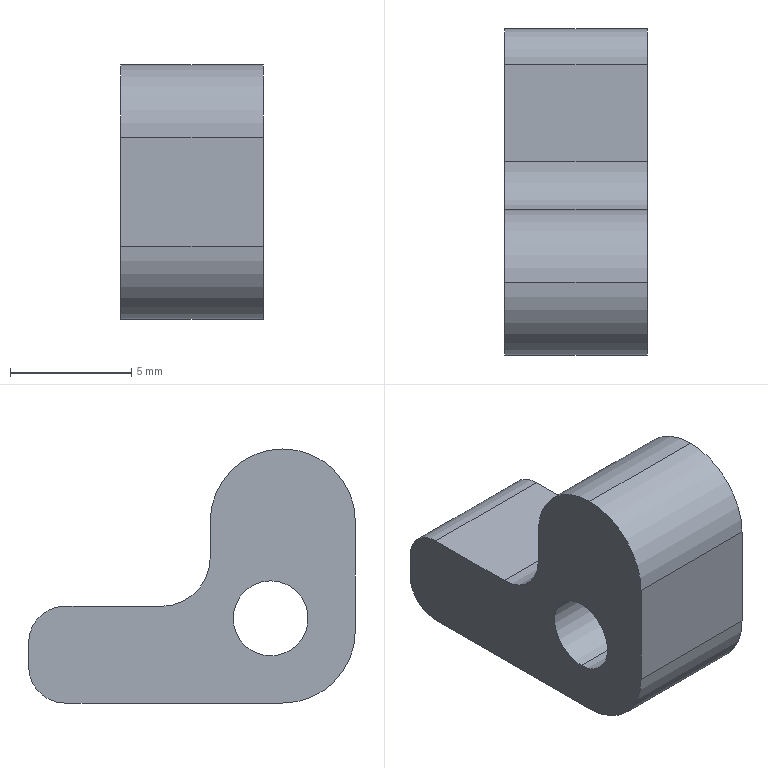Part | STEP file | PN_0095 limit clamp block | 1 solid | 15 faces | box 5.9 x 13.5 x 10.5 mm | volume 469.35 mm3 | cylinder 8 | plane 7 | commonest cylinder face diameters 6 x3 3 x2 3.1 x2 4 x1
STEP:
#1=CARTESIAN_POINT('',(0.,0.,0.));
#2=DIRECTION('',(0.,0.,1.));
#3=DIRECTION('',(1.,0.,0.));
#4=AXIS2_PLACEMENT_3D('',#1,#2,#3);
#5=CARTESIAN_POINT('',(-2.95,0.,1.95));
#6=VERTEX_POINT('',#5);
#7=CARTESIAN_POINT('',(2.95,0.,1.95));
#8=VERTEX_POINT('',#7);
#9=CARTESIAN_POINT('',(-2.95,0.,1.95));
#10=DIRECTION('',(1.,0.,0.));
#11=VECTOR('',#10,1.);
#12=LINE('',#9,#11);
#13=CARTESIAN_POINT('',(-2.95,0.,3.5));
#14=DIRECTION('',(1.,0.,0.));
#15=DIRECTION('',(0.,0.,-1.));
#16=AXIS2_PLACEMENT_3D('',#13,#14,#15);
#17=CYLINDRICAL_SURFACE('',#16,1.55);
#18=CARTESIAN_POINT('',(6.283,0.));
#19=DIRECTION('',(0.,1.));
#20=VECTOR('',#19,1.);
#21=LINE('',#18,#20);
#22=(GEOMETRIC_REPRESENTATION_CONTEXT(2)PARAMETRIC_REPRESENTATION_CONTEXT()REPRESENTATION_CONTEXT('',''));
#23=DEFINITIONAL_REPRESENTATION('',(#21),#22);
#24=PCURVE('',#17,#23);
#25=CARTESIAN_POINT('',(-2.95,0.,3.5));
#26=DIRECTION('',(1.,0.,0.));
#27=DIRECTION('',(0.,0.,-1.));
#28=AXIS2_PLACEMENT_3D('',#25,#26,#27);
#29=CYLINDRICAL_SURFACE('',#28,1.55);
#30=CARTESIAN_POINT('',(0.,0.));
#31=DIRECTION('',(0.,1.));
#32=VECTOR('',#31,1.);
#33=LINE('',#30,#32);
#34=(GEOMETRIC_REPRESENTATION_CONTEXT(2)PARAMETRIC_REPRESENTATION_CONTEXT()REPRESENTATION_CONTEXT('',''));
#35=DEFINITIONAL_REPRESENTATION('',(#33),#34);
#36=PCURVE('',#29,#35);
#37=SURFACE_CURVE('',#12,(#24,#36),.PCURVE_S1.);
#38=EDGE_CURVE('',#6,#8,#37,.T.);
#39=ORIENTED_EDGE('',*,*,#38,.T.);
#40=CARTESIAN_POINT('',(2.95,0.,5.05));
#41=VERTEX_POINT('',#40);
#42=CARTESIAN_POINT('',(2.95,0.,3.5));
#43=DIRECTION('',(1.,0.,0.));
#44=DIRECTION('',(0.,0.,-1.));
#45=AXIS2_PLACEMENT_3D('',#42,#43,#44);
#46=CIRCLE('',#45,1.55);
#47=CARTESIAN_POINT('',(0.,5.9));
#48=DIRECTION('',(1.,0.));
#49=VECTOR('',#48,1.);
#50=LINE('',#47,#49);
#51=(GEOMETRIC_REPRESENTATION_CONTEXT(2)PARAMETRIC_REPRESENTATION_CONTEXT()REPRESENTATION_CONTEXT('',''));
#52=DEFINITIONAL_REPRESENTATION('',(#50),#51);
#53=PCURVE('',#17,#52);
#54=CARTESIAN_POINT('',(2.95,-10.,4.));
#55=DIRECTION('',(-1.,0.,0.));
#56=DIRECTION('',(0.,0.,1.));
#57=AXIS2_PLACEMENT_3D('',#54,#55,#56);
#58=PLANE('',#57);
#59=CARTESIAN_POINT('',(-2.05,10.));
#60=CARTESIAN_POINT('',(-2.05,12.685));
#61=CARTESIAN_POINT('',(0.275,11.342));
#62=CARTESIAN_POINT('',(2.6,10.));
#63=CARTESIAN_POINT('',(0.275,8.658));
#64=CARTESIAN_POINT('',(-2.05,7.315));
#65=CARTESIAN_POINT('',(-2.05,10.));
#66=(BOUNDED_CURVE()B_SPLINE_CURVE(2,(#59,#60,#61,#62,#63,#64,#65),.UNSPECIFIED.,.T.,.F.)B_SPLINE_CURVE_WITH_KNOTS((1,2,2,2,2,1),(-2.094,0.,2.094,4.189,6.283,8.378),.UNSPECIFIED.)CURVE()GEOMETRIC_REPRESENTATION_ITEM()RATIONAL_B_SPLINE_CURVE((1.,0.5,1.,0.5,1.,0.5,1.))REPRESENTATION_ITEM(''));
#67=(GEOMETRIC_REPRESENTATION_CONTEXT(2)PARAMETRIC_REPRESENTATION_CONTEXT()REPRESENTATION_CONTEXT('',''));
#68=DEFINITIONAL_REPRESENTATION('',(#66),#67);
#69=PCURVE('',#58,#68);
#70=SURFACE_CURVE('',#46,(#53,#69),.PCURVE_S1.);
#71=EDGE_CURVE('',#41,#8,#70,.T.);
#72=ORIENTED_EDGE('',*,*,#71,.F.);
#73=CARTESIAN_POINT('',(-2.95,0.,5.05));
#74=VERTEX_POINT('',#73);
#75=CARTESIAN_POINT('',(-2.95,0.,5.05));
#76=DIRECTION('',(1.,0.,0.));
#77=VECTOR('',#76,1.);
#78=LINE('',#75,#77);
#79=CARTESIAN_POINT('',(3.142,0.));
#80=DIRECTION('',(0.,1.));
#81=VECTOR('',#80,1.);
#82=LINE('',#79,#81);
#83=(GEOMETRIC_REPRESENTATION_CONTEXT(2)PARAMETRIC_REPRESENTATION_CONTEXT()REPRESENTATION_CONTEXT('',''));
#84=DEFINITIONAL_REPRESENTATION('',(#82),#83);
#85=PCURVE('',#17,#84);
#86=CARTESIAN_POINT('',(3.142,0.));
#87=DIRECTION('',(0.,1.));
#88=VECTOR('',#87,1.);
#89=LINE('',#86,#88);
#90=(GEOMETRIC_REPRESENTATION_CONTEXT(2)PARAMETRIC_REPRESENTATION_CONTEXT()REPRESENTATION_CONTEXT('',''));
#91=DEFINITIONAL_REPRESENTATION('',(#89),#90);
#92=PCURVE('',#29,#91);
#93=SURFACE_CURVE('',#78,(#85,#92),.PCURVE_S1.);
#94=EDGE_CURVE('',#74,#41,#93,.T.);
#95=ORIENTED_EDGE('',*,*,#94,.F.);
#96=CARTESIAN_POINT('',(-2.95,0.,3.5));
#97=DIRECTION('',(1.,0.,0.));
#98=DIRECTION('',(0.,0.,-1.));
#99=AXIS2_PLACEMENT_3D('',#96,#97,#98);
#100=CIRCLE('',#99,1.55);
#101=CARTESIAN_POINT('',(0.,0.00005));
#102=DIRECTION('',(1.,0.));
#103=VECTOR('',#102,1.);
#104=LINE('',#101,#103);
#105=(GEOMETRIC_REPRESENTATION_CONTEXT(2)PARAMETRIC_REPRESENTATION_CONTEXT()REPRESENTATION_CONTEXT('',''));
#106=DEFINITIONAL_REPRESENTATION('',(#104),#105);
#107=PCURVE('',#17,#106);
#108=CARTESIAN_POINT('',(-2.95,-10.,4.));
#109=DIRECTION('',(1.,0.,0.));
#110=DIRECTION('',(0.,0.,-1.));
#111=AXIS2_PLACEMENT_3D('',#108,#109,#110);
#112=PLANE('',#111);
#113=CARTESIAN_POINT('',(0.5,10.));
#114=DIRECTION('',(1.,0.));
#115=AXIS2_PLACEMENT_2D('',#113,#114);
#116=CIRCLE('',#115,1.55);
#117=(GEOMETRIC_REPRESENTATION_CONTEXT(2)PARAMETRIC_REPRESENTATION_CONTEXT()REPRESENTATION_CONTEXT('',''));
#118=DEFINITIONAL_REPRESENTATION('',(#116),#117);
#119=PCURVE('',#112,#118);
#120=SURFACE_CURVE('',#100,(#107,#119),.PCURVE_S1.);
#121=EDGE_CURVE('',#74,#6,#120,.T.);
#122=ORIENTED_EDGE('',*,*,#121,.T.);
#123=EDGE_LOOP('',(#39,#72,#95,#122));
#124=FACE_BOUND('',#123,.F.);
#125=ADVANCED_FACE('',(#124),#17,.F.);
#126=CARTESIAN_POINT('',(2.95,0.,3.5));
#127=DIRECTION('',(1.,0.,0.));
#128=DIRECTION('',(0.,0.,-1.));
#129=AXIS2_PLACEMENT_3D('',#126,#127,#128);
#130=CIRCLE('',#129,1.55);
#131=CARTESIAN_POINT('',(-2.05,10.));
#132=CARTESIAN_POINT('',(-2.05,12.685));
#133=CARTESIAN_POINT('',(0.275,11.342));
#134=CARTESIAN_POINT('',(2.6,10.));
#135=CARTESIAN_POINT('',(0.275,8.658));
#136=CARTESIAN_POINT('',(-2.05,7.315));
#137=CARTESIAN_POINT('',(-2.05,10.));
#138=(BOUNDED_CURVE()B_SPLINE_CURVE(2,(#131,#132,#133,#134,#135,#136,#137),.UNSPECIFIED.,.T.,.F.)B_SPLINE_CURVE_WITH_KNOTS((1,2,2,2,2,1),(-2.094,0.,2.094,4.189,6.283,8.378),.UNSPECIFIED.)CURVE()GEOMETRIC_REPRESENTATION_ITEM()RATIONAL_B_SPLINE_CURVE((1.,0.5,1.,0.5,1.,0.5,1.))REPRESENTATION_ITEM(''));
#139=(GEOMETRIC_REPRESENTATION_CONTEXT(2)PARAMETRIC_REPRESENTATION_CONTEXT()REPRESENTATION_CONTEXT('',''));
#140=DEFINITIONAL_REPRESENTATION('',(#138),#139);
#141=PCURVE('',#58,#140);
#142=CARTESIAN_POINT('',(0.,5.9));
#143=DIRECTION('',(1.,0.));
#144=VECTOR('',#143,1.);
#145=LINE('',#142,#144);
#146=(GEOMETRIC_REPRESENTATION_CONTEXT(2)PARAMETRIC_REPRESENTATION_CONTEXT()REPRESENTATION_CONTEXT('',''));
#147=DEFINITIONAL_REPRESENTATION('',(#145),#146);
#148=PCURVE('',#29,#147);
#149=SURFACE_CURVE('',#130,(#141,#148),.PCURVE_S1.);
#150=EDGE_CURVE('',#8,#41,#149,.T.);
#151=ORIENTED_EDGE('',*,*,#150,.F.);
#152=ORIENTED_EDGE('',*,*,#71,.F.);
#153=EDGE_LOOP('',(#151,#152));
#154=FACE_BOUND('',#153,.T.);
#155=CARTESIAN_POINT('',(2.95,2.5,7.5));
#156=VERTEX_POINT('',#155);
#157=CARTESIAN_POINT('',(2.95,-0.5,10.5));
#158=VERTEX_POINT('',#157);
#159=CARTESIAN_POINT('',(2.95,-0.5,7.5));
#160=DIRECTION('',(1.,0.,0.));
#161=DIRECTION('',(0.,0.,1.));
#162=AXIS2_PLACEMENT_3D('',#159,#160,#161);
#163=CIRCLE('',#162,3.);
#164=CARTESIAN_POINT('',(6.5,9.5));
#165=CARTESIAN_POINT('',(6.5,4.304));
#166=CARTESIAN_POINT('',(2.,6.902));
#167=CARTESIAN_POINT('',(-2.5,9.5));
#168=CARTESIAN_POINT('',(2.,12.098));
#169=CARTESIAN_POINT('',(6.5,14.696));
#170=CARTESIAN_POINT('',(6.5,9.5));
#171=(BOUNDED_CURVE()B_SPLINE_CURVE(2,(#164,#165,#166,#167,#168,#169,#170),.UNSPECIFIED.,.T.,.F.)B_SPLINE_CURVE_WITH_KNOTS((1,2,2,2,2,1),(-2.094,0.,2.094,4.189,6.283,8.378),.UNSPECIFIED.)CURVE()GEOMETRIC_REPRESENTATION_ITEM()RATIONAL_B_SPLINE_CURVE((1.,0.5,1.,0.5,1.,0.5,1.))REPRESENTATION_ITEM(''));
#172=(GEOMETRIC_REPRESENTATION_CONTEXT(2)PARAMETRIC_REPRESENTATION_CONTEXT()REPRESENTATION_CONTEXT('',''));
#173=DEFINITIONAL_REPRESENTATION('',(#171),#172);
#174=PCURVE('',#58,#173);
#175=CARTESIAN_POINT('',(0.,-0.5,7.5));
#176=DIRECTION('',(-1.,0.,0.));
#177=DIRECTION('',(0.,0.,1.));
#178=AXIS2_PLACEMENT_3D('',#175,#176,#177);
#179=CYLINDRICAL_SURFACE('',#178,3.);
#180=CARTESIAN_POINT('',(6.283,-2.95));
#181=DIRECTION('',(-1.,0.));
#182=VECTOR('',#181,1.);
#183=LINE('',#180,#182);
#184=(GEOMETRIC_REPRESENTATION_CONTEXT(2)PARAMETRIC_REPRESENTATION_CONTEXT()REPRESENTATION_CONTEXT('',''));
#185=DEFINITIONAL_REPRESENTATION('',(#183),#184);
#186=PCURVE('',#179,#185);
#187=SURFACE_CURVE('',#163,(#174,#186),.PCURVE_S1.);
#188=EDGE_CURVE('',#156,#158,#187,.T.);
#189=ORIENTED_EDGE('',*,*,#188,.T.);
#190=CARTESIAN_POINT('',(2.95,-3.5,7.5));
#191=VERTEX_POINT('',#190);
#192=CARTESIAN_POINT('',(2.95,-0.5,7.5));
#193=DIRECTION('',(1.,0.,0.));
#194=DIRECTION('',(0.,0.,1.));
#195=AXIS2_PLACEMENT_3D('',#192,#193,#194);
#196=CIRCLE('',#195,3.);
#197=CARTESIAN_POINT('',(6.5,9.5));
#198=CARTESIAN_POINT('',(6.5,4.304));
#199=CARTESIAN_POINT('',(2.,6.902));
#200=CARTESIAN_POINT('',(-2.5,9.5));
#201=CARTESIAN_POINT('',(2.,12.098));
#202=CARTESIAN_POINT('',(6.5,14.696));
#203=CARTESIAN_POINT('',(6.5,9.5));
#204=(BOUNDED_CURVE()B_SPLINE_CURVE(2,(#197,#198,#199,#200,#201,#202,#203),.UNSPECIFIED.,.T.,.F.)B_SPLINE_CURVE_WITH_KNOTS((1,2,2,2,2,1),(-2.094,0.,2.094,4.189,6.283,8.378),.UNSPECIFIED.)CURVE()GEOMETRIC_REPRESENTATION_ITEM()RATIONAL_B_SPLINE_CURVE((1.,0.5,1.,0.5,1.,0.5,1.))REPRESENTATION_ITEM(''));
#205=(GEOMETRIC_REPRESENTATION_CONTEXT(2)PARAMETRIC_REPRESENTATION_CONTEXT()REPRESENTATION_CONTEXT('',''));
#206=DEFINITIONAL_REPRESENTATION('',(#204),#205);
#207=PCURVE('',#58,#206);
#208=CARTESIAN_POINT('',(0.,-0.5,7.5));
#209=DIRECTION('',(1.,0.,0.));
#210=DIRECTION('',(0.,0.,-1.));
#211=AXIS2_PLACEMENT_3D('',#208,#209,#210);
#212=CYLINDRICAL_SURFACE('',#211,3.);
#213=CARTESIAN_POINT('',(3.142,2.95));
#214=DIRECTION('',(1.,0.));
#215=VECTOR('',#214,1.);
#216=LINE('',#213,#215);
#217=(GEOMETRIC_REPRESENTATION_CONTEXT(2)PARAMETRIC_REPRESENTATION_CONTEXT()REPRESENTATION_CONTEXT('',''));
#218=DEFINITIONAL_REPRESENTATION('',(#216),#217);
#219=PCURVE('',#212,#218);
#220=SURFACE_CURVE('',#196,(#207,#219),.PCURVE_S1.);
#221=EDGE_CURVE('',#158,#191,#220,.T.);
#222=ORIENTED_EDGE('',*,*,#221,.T.);
#223=CARTESIAN_POINT('',(2.95,-3.5,3.));
#224=VERTEX_POINT('',#223);
#225=CARTESIAN_POINT('',(2.95,-3.5,10.5));
#226=DIRECTION('',(0.,0.,-1.));
#227=VECTOR('',#226,1.);
#228=LINE('',#225,#227);
#229=CARTESIAN_POINT('',(6.5,6.5));
#230=DIRECTION('',(-1.,0.));
#231=VECTOR('',#230,1.);
#232=LINE('',#229,#231);
#233=(GEOMETRIC_REPRESENTATION_CONTEXT(2)PARAMETRIC_REPRESENTATION_CONTEXT()REPRESENTATION_CONTEXT('',''));
#234=DEFINITIONAL_REPRESENTATION('',(#232),#233);
#235=PCURVE('',#58,#234);
#236=CARTESIAN_POINT('',(-2.95,-3.5,10.5));
#237=DIRECTION('',(0.,1.,0.));
#238=DIRECTION('',(0.,0.,1.));
#239=AXIS2_PLACEMENT_3D('',#236,#237,#238);
#240=PLANE('',#239);
#241=CARTESIAN_POINT('',(0.,5.9));
#242=DIRECTION('',(-1.,0.));
#243=VECTOR('',#242,1.);
#244=LINE('',#241,#243);
#245=(GEOMETRIC_REPRESENTATION_CONTEXT(2)PARAMETRIC_REPRESENTATION_CONTEXT()REPRESENTATION_CONTEXT('',''));
#246=DEFINITIONAL_REPRESENTATION('',(#244),#245);
#247=PCURVE('',#240,#246);
#248=SURFACE_CURVE('',#228,(#235,#247),.PCURVE_S1.);
#249=EDGE_CURVE('',#191,#224,#248,.T.);
#250=ORIENTED_EDGE('',*,*,#249,.T.);
#251=CARTESIAN_POINT('',(2.95,-0.5,0.));
#252=VERTEX_POINT('',#251);
#253=CARTESIAN_POINT('',(2.95,-0.5,3.));
#254=DIRECTION('',(1.,0.,0.));
#255=DIRECTION('',(0.,0.,1.));
#256=AXIS2_PLACEMENT_3D('',#253,#254,#255);
#257=CIRCLE('',#256,3.);
#258=CARTESIAN_POINT('',(2.,9.5));
#259=CARTESIAN_POINT('',(2.,4.304));
#260=CARTESIAN_POINT('',(-2.5,6.902));
#261=CARTESIAN_POINT('',(-7.,9.5));
#262=CARTESIAN_POINT('',(-2.5,12.098));
#263=CARTESIAN_POINT('',(2.,14.696));
#264=CARTESIAN_POINT('',(2.,9.5));
#265=(BOUNDED_CURVE()B_SPLINE_CURVE(2,(#258,#259,#260,#261,#262,#263,#264),.UNSPECIFIED.,.T.,.F.)B_SPLINE_CURVE_WITH_KNOTS((1,2,2,2,2,1),(-2.094,0.,2.094,4.189,6.283,8.378),.UNSPECIFIED.)CURVE()GEOMETRIC_REPRESENTATION_ITEM()RATIONAL_B_SPLINE_CURVE((1.,0.5,1.,0.5,1.,0.5,1.))REPRESENTATION_ITEM(''));
#266=(GEOMETRIC_REPRESENTATION_CONTEXT(2)PARAMETRIC_REPRESENTATION_CONTEXT()REPRESENTATION_CONTEXT('',''));
#267=DEFINITIONAL_REPRESENTATION('',(#265),#266);
#268=PCURVE('',#58,#267);
#269=CARTESIAN_POINT('',(0.,-0.5,3.));
#270=DIRECTION('',(1.,0.,0.));
#271=DIRECTION('',(0.,0.,-1.));
#272=AXIS2_PLACEMENT_3D('',#269,#270,#271);
#273=CYLINDRICAL_SURFACE('',#272,3.);
#274=CARTESIAN_POINT('',(3.142,2.95));
#275=DIRECTION('',(1.,0.));
#276=VECTOR('',#275,1.);
#277=LINE('',#274,#276);
#278=(GEOMETRIC_REPRESENTATION_CONTEXT(2)PARAMETRIC_REPRESENTATION_CONTEXT()REPRESENTATION_CONTEXT('',''));
#279=DEFINITIONAL_REPRESENTATION('',(#277),#278);
#280=PCURVE('',#273,#279);
#281=SURFACE_CURVE('',#257,(#268,#280),.PCURVE_S1.);
#282=EDGE_CURVE('',#224,#252,#281,.T.);
#283=ORIENTED_EDGE('',*,*,#282,.T.);
#284=CARTESIAN_POINT('',(2.95,8.5,0.));
#285=VERTEX_POINT('',#284);
#286=CARTESIAN_POINT('',(2.95,-10.,0.));
#287=DIRECTION('',(0.,1.,0.));
#288=VECTOR('',#287,1.);
#289=LINE('',#286,#288);
#290=CARTESIAN_POINT('',(-4.,0.));
#291=DIRECTION('',(0.,1.));
#292=VECTOR('',#291,1.);
#293=LINE('',#290,#292);
#294=(GEOMETRIC_REPRESENTATION_CONTEXT(2)PARAMETRIC_REPRESENTATION_CONTEXT()REPRESENTATION_CONTEXT('',''));
#295=DEFINITIONAL_REPRESENTATION('',(#293),#294);
#296=PCURVE('',#58,#295);
#297=CARTESIAN_POINT('',(0.,0.,0.));
#298=DIRECTION('',(0.,0.,-1.));
#299=DIRECTION('',(-1.,0.,0.));
#300=AXIS2_PLACEMENT_3D('',#297,#298,#299);
#301=PLANE('',#300);
#302=CARTESIAN_POINT('',(-2.95,-10.));
#303=DIRECTION('',(0.,1.));
#304=VECTOR('',#303,1.);
#305=LINE('',#302,#304);
#306=(GEOMETRIC_REPRESENTATION_CONTEXT(2)PARAMETRIC_REPRESENTATION_CONTEXT()REPRESENTATION_CONTEXT('',''));
#307=DEFINITIONAL_REPRESENTATION('',(#305),#306);
#308=PCURVE('',#301,#307);
#309=SURFACE_CURVE('',#289,(#296,#308),.PCURVE_S1.);
#310=EDGE_CURVE('',#252,#285,#309,.T.);
#311=ORIENTED_EDGE('',*,*,#310,.T.);
#312=CARTESIAN_POINT('',(2.95,10.,1.5));
#313=VERTEX_POINT('',#312);
#314=CARTESIAN_POINT('',(2.95,8.5,1.5));
#315=DIRECTION('',(1.,0.,0.));
#316=DIRECTION('',(0.,0.,1.));
#317=AXIS2_PLACEMENT_3D('',#314,#315,#316);
#318=CIRCLE('',#317,1.5);
#319=CARTESIAN_POINT('',(-1.,18.5));
#320=CARTESIAN_POINT('',(-1.,15.902));
#321=CARTESIAN_POINT('',(-3.25,17.201));
#322=CARTESIAN_POINT('',(-5.5,18.5));
#323=CARTESIAN_POINT('',(-3.25,19.799));
#324=CARTESIAN_POINT('',(-1.,21.098));
#325=CARTESIAN_POINT('',(-1.,18.5));
#326=(BOUNDED_CURVE()B_SPLINE_CURVE(2,(#319,#320,#321,#322,#323,#324,#325),.UNSPECIFIED.,.T.,.F.)B_SPLINE_CURVE_WITH_KNOTS((1,2,2,2,2,1),(-2.094,0.,2.094,4.189,6.283,8.378),.UNSPECIFIED.)CURVE()GEOMETRIC_REPRESENTATION_ITEM()RATIONAL_B_SPLINE_CURVE((1.,0.5,1.,0.5,1.,0.5,1.))REPRESENTATION_ITEM(''));
#327=(GEOMETRIC_REPRESENTATION_CONTEXT(2)PARAMETRIC_REPRESENTATION_CONTEXT()REPRESENTATION_CONTEXT('',''));
#328=DEFINITIONAL_REPRESENTATION('',(#326),#327);
#329=PCURVE('',#58,#328);
#330=CARTESIAN_POINT('',(-2.95,8.5,1.5));
#331=DIRECTION('',(1.,0.,0.));
#332=DIRECTION('',(0.,0.,-1.));
#333=AXIS2_PLACEMENT_3D('',#330,#331,#332);
#334=CYLINDRICAL_SURFACE('',#333,1.5);
#335=CARTESIAN_POINT('',(-3.142,5.9));
#336=DIRECTION('',(1.,0.));
#337=VECTOR('',#336,1.);
#338=LINE('',#335,#337);
#339=(GEOMETRIC_REPRESENTATION_CONTEXT(2)PARAMETRIC_REPRESENTATION_CONTEXT()REPRESENTATION_CONTEXT('',''));
#340=DEFINITIONAL_REPRESENTATION('',(#338),#339);
#341=PCURVE('',#334,#340);
#342=SURFACE_CURVE('',#318,(#329,#341),.PCURVE_S1.);
#343=EDGE_CURVE('',#285,#313,#342,.T.);
#344=ORIENTED_EDGE('',*,*,#343,.T.);
#345=CARTESIAN_POINT('',(2.95,10.,2.5));
#346=VERTEX_POINT('',#345);
#347=CARTESIAN_POINT('',(2.95,10.,4.));
#348=DIRECTION('',(0.,0.,-1.));
#349=VECTOR('',#348,1.);
#350=LINE('',#347,#349);
#351=CARTESIAN_POINT('',(0.,20.));
#352=DIRECTION('',(-1.,0.));
#353=VECTOR('',#352,1.);
#354=LINE('',#351,#353);
#355=(GEOMETRIC_REPRESENTATION_CONTEXT(2)PARAMETRIC_REPRESENTATION_CONTEXT()REPRESENTATION_CONTEXT('',''));
#356=DEFINITIONAL_REPRESENTATION('',(#354),#355);
#357=PCURVE('',#58,#356);
#358=CARTESIAN_POINT('',(-2.95,10.,4.));
#359=DIRECTION('',(0.,-1.,0.));
#360=DIRECTION('',(0.,0.,-1.));
#361=AXIS2_PLACEMENT_3D('',#358,#359,#360);
#362=PLANE('',#361);
#363=CARTESIAN_POINT('',(0.,5.9));
#364=DIRECTION('',(1.,0.));
#365=VECTOR('',#364,1.);
#366=LINE('',#363,#365);
#367=(GEOMETRIC_REPRESENTATION_CONTEXT(2)PARAMETRIC_REPRESENTATION_CONTEXT()REPRESENTATION_CONTEXT('',''));
#368=DEFINITIONAL_REPRESENTATION('',(#366),#367);
#369=PCURVE('',#362,#368);
#370=SURFACE_CURVE('',#350,(#357,#369),.PCURVE_S1.);
#371=EDGE_CURVE('',#346,#313,#370,.T.);
#372=ORIENTED_EDGE('',*,*,#371,.F.);
#373=CARTESIAN_POINT('',(2.95,8.5,4.));
#374=VERTEX_POINT('',#373);
#375=CARTESIAN_POINT('',(2.95,8.5,2.5));
#376=DIRECTION('',(1.,0.,0.));
#377=DIRECTION('',(0.,0.,1.));
#378=AXIS2_PLACEMENT_3D('',#375,#376,#377);
#379=CIRCLE('',#378,1.5);
#380=CARTESIAN_POINT('',(0.,18.5));
#381=CARTESIAN_POINT('',(0.,15.902));
#382=CARTESIAN_POINT('',(-2.25,17.201));
#383=CARTESIAN_POINT('',(-4.5,18.5));
#384=CARTESIAN_POINT('',(-2.25,19.799));
#385=CARTESIAN_POINT('',(0.,21.098));
#386=CARTESIAN_POINT('',(0.,18.5));
#387=(BOUNDED_CURVE()B_SPLINE_CURVE(2,(#380,#381,#382,#383,#384,#385,#386),.UNSPECIFIED.,.T.,.F.)B_SPLINE_CURVE_WITH_KNOTS((1,2,2,2,2,1),(-2.094,0.,2.094,4.189,6.283,8.378),.UNSPECIFIED.)CURVE()GEOMETRIC_REPRESENTATION_ITEM()RATIONAL_B_SPLINE_CURVE((1.,0.5,1.,0.5,1.,0.5,1.))REPRESENTATION_ITEM(''));
#388=(GEOMETRIC_REPRESENTATION_CONTEXT(2)PARAMETRIC_REPRESENTATION_CONTEXT()REPRESENTATION_CONTEXT('',''));
#389=DEFINITIONAL_REPRESENTATION('',(#387),#388);
#390=PCURVE('',#58,#389);
#391=CARTESIAN_POINT('',(0.,8.5,2.5));
#392=DIRECTION('',(-1.,0.,0.));
#393=DIRECTION('',(0.,0.,1.));
#394=AXIS2_PLACEMENT_3D('',#391,#392,#393);
#395=CYLINDRICAL_SURFACE('',#394,1.5);
#396=CARTESIAN_POINT('',(6.283,-2.95));
#397=DIRECTION('',(-1.,0.));
#398=VECTOR('',#397,1.);
#399=LINE('',#396,#398);
#400=(GEOMETRIC_REPRESENTATION_CONTEXT(2)PARAMETRIC_REPRESENTATION_CONTEXT()REPRESENTATION_CONTEXT('',''));
#401=DEFINITIONAL_REPRESENTATION('',(#399),#400);
#402=PCURVE('',#395,#401);
#403=SURFACE_CURVE('',#379,(#390,#402),.PCURVE_S1.);
#404=EDGE_CURVE('',#346,#374,#403,.T.);
#405=ORIENTED_EDGE('',*,*,#404,.T.);
#406=CARTESIAN_POINT('',(2.95,4.5,4.));
#407=VERTEX_POINT('',#406);
#408=CARTESIAN_POINT('',(2.95,-10.,4.));
#409=DIRECTION('',(0.,1.,0.));
#410=VECTOR('',#409,1.);
#411=LINE('',#408,#410);
#412=CARTESIAN_POINT('',(0.,0.));
#413=DIRECTION('',(0.,1.));
#414=VECTOR('',#413,1.);
#415=LINE('',#412,#414);
#416=(GEOMETRIC_REPRESENTATION_CONTEXT(2)PARAMETRIC_REPRESENTATION_CONTEXT()REPRESENTATION_CONTEXT('',''));
#417=DEFINITIONAL_REPRESENTATION('',(#415),#416);
#418=PCURVE('',#58,#417);
#419=CARTESIAN_POINT('',(0.,0.,4.));
#420=DIRECTION('',(0.,0.,-1.));
#421=DIRECTION('',(-1.,0.,0.));
#422=AXIS2_PLACEMENT_3D('',#419,#420,#421);
#423=PLANE('',#422);
#424=CARTESIAN_POINT('',(-2.95,-10.));
#425=DIRECTION('',(0.,1.));
#426=VECTOR('',#425,1.);
#427=LINE('',#424,#426);
#428=(GEOMETRIC_REPRESENTATION_CONTEXT(2)PARAMETRIC_REPRESENTATION_CONTEXT()REPRESENTATION_CONTEXT('',''));
#429=DEFINITIONAL_REPRESENTATION('',(#427),#428);
#430=PCURVE('',#423,#429);
#431=SURFACE_CURVE('',#411,(#418,#430),.PCURVE_S1.);
#432=EDGE_CURVE('',#407,#374,#431,.T.);
#433=ORIENTED_EDGE('',*,*,#432,.F.);
#434=CARTESIAN_POINT('',(2.95,2.5,6.));
#435=VERTEX_POINT('',#434);
#436=CARTESIAN_POINT('',(2.95,4.5,6.));
#437=DIRECTION('',(-1.,0.,0.));
#438=DIRECTION('',(0.,0.,1.));
#439=AXIS2_PLACEMENT_3D('',#436,#437,#438);
#440=CIRCLE('',#439,2.);
#441=CARTESIAN_POINT('',(2.,14.5));
#442=DIRECTION('',(1.,0.));
#443=AXIS2_PLACEMENT_2D('',#441,#442);
#444=CIRCLE('',#443,2.);
#445=(GEOMETRIC_REPRESENTATION_CONTEXT(2)PARAMETRIC_REPRESENTATION_CONTEXT()REPRESENTATION_CONTEXT('',''));
#446=DEFINITIONAL_REPRESENTATION('',(#444),#445);
#447=PCURVE('',#58,#446);
#448=CARTESIAN_POINT('',(-2.95,4.5,6.));
#449=DIRECTION('',(1.,0.,0.));
#450=DIRECTION('',(0.,0.,-1.));
#451=AXIS2_PLACEMENT_3D('',#448,#449,#450);
#452=CYLINDRICAL_SURFACE('',#451,2.);
#453=CARTESIAN_POINT('',(9.425,5.9));
#454=DIRECTION('',(-1.,0.));
#455=VECTOR('',#454,1.);
#456=LINE('',#453,#455);
#457=(GEOMETRIC_REPRESENTATION_CONTEXT(2)PARAMETRIC_REPRESENTATION_CONTEXT()REPRESENTATION_CONTEXT('',''));
#458=DEFINITIONAL_REPRESENTATION('',(#456),#457);
#459=PCURVE('',#452,#458);
#460=SURFACE_CURVE('',#440,(#447,#459),.PCURVE_S1.);
#461=EDGE_CURVE('',#407,#435,#460,.T.);
#462=ORIENTED_EDGE('',*,*,#461,.T.);
#463=CARTESIAN_POINT('',(2.95,2.5,10.5));
#464=DIRECTION('',(0.,0.,-1.));
#465=VECTOR('',#464,1.);
#466=LINE('',#463,#465);
#467=CARTESIAN_POINT('',(6.5,12.5));
#468=DIRECTION('',(-1.,0.));
#469=VECTOR('',#468,1.);
#470=LINE('',#467,#469);
#471=(GEOMETRIC_REPRESENTATION_CONTEXT(2)PARAMETRIC_REPRESENTATION_CONTEXT()REPRESENTATION_CONTEXT('',''));
#472=DEFINITIONAL_REPRESENTATION('',(#470),#471);
#473=PCURVE('',#58,#472);
#474=CARTESIAN_POINT('',(-2.95,2.5,10.5));
#475=DIRECTION('',(0.,-1.,0.));
#476=DIRECTION('',(0.,0.,-1.));
#477=AXIS2_PLACEMENT_3D('',#474,#475,#476);
#478=PLANE('',#477);
#479=CARTESIAN_POINT('',(0.,5.9));
#480=DIRECTION('',(1.,0.));
#481=VECTOR('',#480,1.);
#482=LINE('',#479,#481);
#483=(GEOMETRIC_REPRESENTATION_CONTEXT(2)PARAMETRIC_REPRESENTATION_CONTEXT()REPRESENTATION_CONTEXT('',''));
#484=DEFINITIONAL_REPRESENTATION('',(#482),#483);
#485=PCURVE('',#478,#484);
#486=SURFACE_CURVE('',#466,(#473,#485),.PCURVE_S1.);
#487=EDGE_CURVE('',#156,#435,#486,.T.);
#488=ORIENTED_EDGE('',*,*,#487,.F.);
#489=EDGE_LOOP('',(#189,#222,#250,#283,#311,#344,#372,#405,#433,#462,#488));
#490=FACE_BOUND('',#489,.T.);
#491=ADVANCED_FACE('',(#154,#490),#58,.F.);
#492=CARTESIAN_POINT('',(-2.95,0.,3.5));
#493=DIRECTION('',(1.,0.,0.));
#494=DIRECTION('',(0.,0.,-1.));
#495=AXIS2_PLACEMENT_3D('',#492,#493,#494);
#496=CIRCLE('',#495,1.55);
#497=CARTESIAN_POINT('',(0.5,10.));
#498=DIRECTION('',(1.,0.));
#499=AXIS2_PLACEMENT_2D('',#497,#498);
#500=CIRCLE('',#499,1.55);
#501=(GEOMETRIC_REPRESENTATION_CONTEXT(2)PARAMETRIC_REPRESENTATION_CONTEXT()REPRESENTATION_CONTEXT('',''));
#502=DEFINITIONAL_REPRESENTATION('',(#500),#501);
#503=PCURVE('',#112,#502);
#504=CARTESIAN_POINT('',(0.,0.00005));
#505=DIRECTION('',(1.,0.));
#506=VECTOR('',#505,1.);
#507=LINE('',#504,#506);
#508=(GEOMETRIC_REPRESENTATION_CONTEXT(2)PARAMETRIC_REPRESENTATION_CONTEXT()REPRESENTATION_CONTEXT('',''));
#509=DEFINITIONAL_REPRESENTATION('',(#507),#508);
#510=PCURVE('',#29,#509);
#511=SURFACE_CURVE('',#496,(#503,#510),.PCURVE_S1.);
#512=EDGE_CURVE('',#6,#74,#511,.T.);
#513=ORIENTED_EDGE('',*,*,#512,.T.);
#514=ORIENTED_EDGE('',*,*,#121,.T.);
#515=EDGE_LOOP('',(#513,#514));
#516=FACE_BOUND('',#515,.T.);
#517=CARTESIAN_POINT('',(-2.95,-3.5,7.5));
#518=VERTEX_POINT('',#517);
#519=CARTESIAN_POINT('',(-2.95,-3.5,3.));
#520=VERTEX_POINT('',#519);
#521=CARTESIAN_POINT('',(-2.95,-3.5,10.5));
#522=DIRECTION('',(0.,0.,-1.));
#523=VECTOR('',#522,1.);
#524=LINE('',#521,#523);
#525=CARTESIAN_POINT('',(-6.5,6.5));
#526=DIRECTION('',(1.,0.));
#527=VECTOR('',#526,1.);
#528=LINE('',#525,#527);
#529=(GEOMETRIC_REPRESENTATION_CONTEXT(2)PARAMETRIC_REPRESENTATION_CONTEXT()REPRESENTATION_CONTEXT('',''));
#530=DEFINITIONAL_REPRESENTATION('',(#528),#529);
#531=PCURVE('',#112,#530);
#532=CARTESIAN_POINT('',(0.,0.));
#533=DIRECTION('',(-1.,0.));
#534=VECTOR('',#533,1.);
#535=LINE('',#532,#534);
#536=(GEOMETRIC_REPRESENTATION_CONTEXT(2)PARAMETRIC_REPRESENTATION_CONTEXT()REPRESENTATION_CONTEXT('',''));
#537=DEFINITIONAL_REPRESENTATION('',(#535),#536);
#538=PCURVE('',#240,#537);
#539=SURFACE_CURVE('',#524,(#531,#538),.PCURVE_S1.);
#540=EDGE_CURVE('',#518,#520,#539,.T.);
#541=ORIENTED_EDGE('',*,*,#540,.F.);
#542=CARTESIAN_POINT('',(-2.95,-0.5,10.5));
#543=VERTEX_POINT('',#542);
#544=CARTESIAN_POINT('',(-2.95,-0.5,7.5));
#545=DIRECTION('',(-1.,0.,0.));
#546=DIRECTION('',(0.,0.,-1.));
#547=AXIS2_PLACEMENT_3D('',#544,#545,#546);
#548=CIRCLE('',#547,3.);
#549=CARTESIAN_POINT('',(-0.5,9.5));
#550=CARTESIAN_POINT('',(-0.5,4.304));
#551=CARTESIAN_POINT('',(-5.,6.902));
#552=CARTESIAN_POINT('',(-9.5,9.5));
#553=CARTESIAN_POINT('',(-5.,12.098));
#554=CARTESIAN_POINT('',(-0.5,14.696));
#555=CARTESIAN_POINT('',(-0.5,9.5));
#556=(BOUNDED_CURVE()B_SPLINE_CURVE(2,(#549,#550,#551,#552,#553,#554,#555),.UNSPECIFIED.,.T.,.F.)B_SPLINE_CURVE_WITH_KNOTS((1,2,2,2,2,1),(-2.094,0.,2.094,4.189,6.283,8.378),.UNSPECIFIED.)CURVE()GEOMETRIC_REPRESENTATION_ITEM()RATIONAL_B_SPLINE_CURVE((1.,0.5,1.,0.5,1.,0.5,1.))REPRESENTATION_ITEM(''));
#557=(GEOMETRIC_REPRESENTATION_CONTEXT(2)PARAMETRIC_REPRESENTATION_CONTEXT()REPRESENTATION_CONTEXT('',''));
#558=DEFINITIONAL_REPRESENTATION('',(#556),#557);
#559=PCURVE('',#112,#558);
#560=CARTESIAN_POINT('',(6.283,-2.95));
#561=DIRECTION('',(-1.,0.));
#562=VECTOR('',#561,1.);
#563=LINE('',#560,#562);
#564=(GEOMETRIC_REPRESENTATION_CONTEXT(2)PARAMETRIC_REPRESENTATION_CONTEXT()REPRESENTATION_CONTEXT('',''));
#565=DEFINITIONAL_REPRESENTATION('',(#563),#564);
#566=PCURVE('',#212,#565);
#567=SURFACE_CURVE('',#548,(#559,#566),.PCURVE_S1.);
#568=EDGE_CURVE('',#518,#543,#567,.T.);
#569=ORIENTED_EDGE('',*,*,#568,.T.);
#570=CARTESIAN_POINT('',(-2.95,2.5,7.5));
#571=VERTEX_POINT('',#570);
#572=CARTESIAN_POINT('',(-2.95,-0.5,7.5));
#573=DIRECTION('',(-1.,0.,0.));
#574=DIRECTION('',(0.,0.,-1.));
#575=AXIS2_PLACEMENT_3D('',#572,#573,#574);
#576=CIRCLE('',#575,3.);
#577=CARTESIAN_POINT('',(-0.5,9.5));
#578=CARTESIAN_POINT('',(-0.5,4.304));
#579=CARTESIAN_POINT('',(-5.,6.902));
#580=CARTESIAN_POINT('',(-9.5,9.5));
#581=CARTESIAN_POINT('',(-5.,12.098));
#582=CARTESIAN_POINT('',(-0.5,14.696));
#583=CARTESIAN_POINT('',(-0.5,9.5));
#584=(BOUNDED_CURVE()B_SPLINE_CURVE(2,(#577,#578,#579,#580,#581,#582,#583),.UNSPECIFIED.,.T.,.F.)B_SPLINE_CURVE_WITH_KNOTS((1,2,2,2,2,1),(-2.094,0.,2.094,4.189,6.283,8.378),.UNSPECIFIED.)CURVE()GEOMETRIC_REPRESENTATION_ITEM()RATIONAL_B_SPLINE_CURVE((1.,0.5,1.,0.5,1.,0.5,1.))REPRESENTATION_ITEM(''));
#585=(GEOMETRIC_REPRESENTATION_CONTEXT(2)PARAMETRIC_REPRESENTATION_CONTEXT()REPRESENTATION_CONTEXT('',''));
#586=DEFINITIONAL_REPRESENTATION('',(#584),#585);
#587=PCURVE('',#112,#586);
#588=CARTESIAN_POINT('',(-3.142,2.95));
#589=DIRECTION('',(1.,0.));
#590=VECTOR('',#589,1.);
#591=LINE('',#588,#590);
#592=(GEOMETRIC_REPRESENTATION_CONTEXT(2)PARAMETRIC_REPRESENTATION_CONTEXT()REPRESENTATION_CONTEXT('',''));
#593=DEFINITIONAL_REPRESENTATION('',(#591),#592);
#594=PCURVE('',#179,#593);
#595=SURFACE_CURVE('',#576,(#587,#594),.PCURVE_S1.);
#596=EDGE_CURVE('',#543,#571,#595,.T.);
#597=ORIENTED_EDGE('',*,*,#596,.T.);
#598=CARTESIAN_POINT('',(-2.95,2.5,6.));
#599=VERTEX_POINT('',#598);
#600=CARTESIAN_POINT('',(-2.95,2.5,10.5));
#601=DIRECTION('',(0.,0.,-1.));
#602=VECTOR('',#601,1.);
#603=LINE('',#600,#602);
#604=CARTESIAN_POINT('',(-6.5,12.5));
#605=DIRECTION('',(1.,0.));
#606=VECTOR('',#605,1.);
#607=LINE('',#604,#606);
#608=(GEOMETRIC_REPRESENTATION_CONTEXT(2)PARAMETRIC_REPRESENTATION_CONTEXT()REPRESENTATION_CONTEXT('',''));
#609=DEFINITIONAL_REPRESENTATION('',(#607),#608);
#610=PCURVE('',#112,#609);
#611=CARTESIAN_POINT('',(0.,0.));
#612=DIRECTION('',(1.,0.));
#613=VECTOR('',#612,1.);
#614=LINE('',#611,#613);
#615=(GEOMETRIC_REPRESENTATION_CONTEXT(2)PARAMETRIC_REPRESENTATION_CONTEXT()REPRESENTATION_CONTEXT('',''));
#616=DEFINITIONAL_REPRESENTATION('',(#614),#615);
#617=PCURVE('',#478,#616);
#618=SURFACE_CURVE('',#603,(#610,#617),.PCURVE_S1.);
#619=EDGE_CURVE('',#571,#599,#618,.T.);
#620=ORIENTED_EDGE('',*,*,#619,.T.);
#621=CARTESIAN_POINT('',(-2.95,4.5,4.));
#622=VERTEX_POINT('',#621);
#623=CARTESIAN_POINT('',(-2.95,4.5,6.));
#624=DIRECTION('',(1.,0.,0.));
#625=DIRECTION('',(0.,0.,-1.));
#626=AXIS2_PLACEMENT_3D('',#623,#624,#625);
#627=CIRCLE('',#626,2.);
#628=CARTESIAN_POINT('',(-2.,14.5));
#629=DIRECTION('',(1.,0.));
#630=AXIS2_PLACEMENT_2D('',#628,#629);
#631=CIRCLE('',#630,2.);
#632=(GEOMETRIC_REPRESENTATION_CONTEXT(2)PARAMETRIC_REPRESENTATION_CONTEXT()REPRESENTATION_CONTEXT('',''));
#633=DEFINITIONAL_REPRESENTATION('',(#631),#632);
#634=PCURVE('',#112,#633);
#635=CARTESIAN_POINT('',(0.,0.));
#636=DIRECTION('',(1.,0.));
#637=VECTOR('',#636,1.);
#638=LINE('',#635,#637);
#639=(GEOMETRIC_REPRESENTATION_CONTEXT(2)PARAMETRIC_REPRESENTATION_CONTEXT()REPRESENTATION_CONTEXT('',''));
#640=DEFINITIONAL_REPRESENTATION('',(#638),#639);
#641=PCURVE('',#452,#640);
#642=SURFACE_CURVE('',#627,(#634,#641),.PCURVE_S1.);
#643=EDGE_CURVE('',#599,#622,#642,.T.);
#644=ORIENTED_EDGE('',*,*,#643,.T.);
#645=CARTESIAN_POINT('',(-2.95,8.5,4.));
#646=VERTEX_POINT('',#645);
#647=CARTESIAN_POINT('',(-2.95,-10.,4.));
#648=DIRECTION('',(0.,-1.,0.));
#649=VECTOR('',#648,1.);
#650=LINE('',#647,#649);
#651=CARTESIAN_POINT('',(0.,0.));
#652=DIRECTION('',(0.,-1.));
#653=VECTOR('',#652,1.);
#654=LINE('',#651,#653);
#655=(GEOMETRIC_REPRESENTATION_CONTEXT(2)PARAMETRIC_REPRESENTATION_CONTEXT()REPRESENTATION_CONTEXT('',''));
#656=DEFINITIONAL_REPRESENTATION('',(#654),#655);
#657=PCURVE('',#112,#656);
#658=CARTESIAN_POINT('',(2.95,-10.));
#659=DIRECTION('',(0.,-1.));
#660=VECTOR('',#659,1.);
#661=LINE('',#658,#660);
#662=(GEOMETRIC_REPRESENTATION_CONTEXT(2)PARAMETRIC_REPRESENTATION_CONTEXT()REPRESENTATION_CONTEXT('',''));
#663=DEFINITIONAL_REPRESENTATION('',(#661),#662);
#664=PCURVE('',#423,#663);
#665=SURFACE_CURVE('',#650,(#657,#664),.PCURVE_S1.);
#666=EDGE_CURVE('',#646,#622,#665,.T.);
#667=ORIENTED_EDGE('',*,*,#666,.F.);
#668=CARTESIAN_POINT('',(-2.95,10.,2.5));
#669=VERTEX_POINT('',#668);
#670=CARTESIAN_POINT('',(-2.95,8.5,2.5));
#671=DIRECTION('',(-1.,0.,0.));
#672=DIRECTION('',(0.,0.,-1.));
#673=AXIS2_PLACEMENT_3D('',#670,#671,#672);
#674=CIRCLE('',#673,1.5);
#675=CARTESIAN_POINT('',(3.,18.5));
#676=CARTESIAN_POINT('',(3.,15.902));
#677=CARTESIAN_POINT('',(0.75,17.201));
#678=CARTESIAN_POINT('',(-1.5,18.5));
#679=CARTESIAN_POINT('',(0.75,19.799));
#680=CARTESIAN_POINT('',(3.,21.098));
#681=CARTESIAN_POINT('',(3.,18.5));
#682=(BOUNDED_CURVE()B_SPLINE_CURVE(2,(#675,#676,#677,#678,#679,#680,#681),.UNSPECIFIED.,.T.,.F.)B_SPLINE_CURVE_WITH_KNOTS((1,2,2,2,2,1),(-2.094,0.,2.094,4.189,6.283,8.378),.UNSPECIFIED.)CURVE()GEOMETRIC_REPRESENTATION_ITEM()RATIONAL_B_SPLINE_CURVE((1.,0.5,1.,0.5,1.,0.5,1.))REPRESENTATION_ITEM(''));
#683=(GEOMETRIC_REPRESENTATION_CONTEXT(2)PARAMETRIC_REPRESENTATION_CONTEXT()REPRESENTATION_CONTEXT('',''));
#684=DEFINITIONAL_REPRESENTATION('',(#682),#683);
#685=PCURVE('',#112,#684);
#686=CARTESIAN_POINT('',(-3.142,2.95));
#687=DIRECTION('',(1.,0.));
#688=VECTOR('',#687,1.);
#689=LINE('',#686,#688);
#690=(GEOMETRIC_REPRESENTATION_CONTEXT(2)PARAMETRIC_REPRESENTATION_CONTEXT()REPRESENTATION_CONTEXT('',''));
#691=DEFINITIONAL_REPRESENTATION('',(#689),#690);
#692=PCURVE('',#395,#691);
#693=SURFACE_CURVE('',#674,(#685,#692),.PCURVE_S1.);
#694=EDGE_CURVE('',#646,#669,#693,.T.);
#695=ORIENTED_EDGE('',*,*,#694,.T.);
#696=CARTESIAN_POINT('',(-2.95,10.,1.5));
#697=VERTEX_POINT('',#696);
#698=CARTESIAN_POINT('',(-2.95,10.,4.));
#699=DIRECTION('',(0.,0.,-1.));
#700=VECTOR('',#699,1.);
#701=LINE('',#698,#700);
#702=CARTESIAN_POINT('',(0.,20.));
#703=DIRECTION('',(1.,0.));
#704=VECTOR('',#703,1.);
#705=LINE('',#702,#704);
#706=(GEOMETRIC_REPRESENTATION_CONTEXT(2)PARAMETRIC_REPRESENTATION_CONTEXT()REPRESENTATION_CONTEXT('',''));
#707=DEFINITIONAL_REPRESENTATION('',(#705),#706);
#708=PCURVE('',#112,#707);
#709=CARTESIAN_POINT('',(0.,0.));
#710=DIRECTION('',(1.,0.));
#711=VECTOR('',#710,1.);
#712=LINE('',#709,#711);
#713=(GEOMETRIC_REPRESENTATION_CONTEXT(2)PARAMETRIC_REPRESENTATION_CONTEXT()REPRESENTATION_CONTEXT('',''));
#714=DEFINITIONAL_REPRESENTATION('',(#712),#713);
#715=PCURVE('',#362,#714);
#716=SURFACE_CURVE('',#701,(#708,#715),.PCURVE_S1.);
#717=EDGE_CURVE('',#669,#697,#716,.T.);
#718=ORIENTED_EDGE('',*,*,#717,.T.);
#719=CARTESIAN_POINT('',(-2.95,8.5,0.));
#720=VERTEX_POINT('',#719);
#721=CARTESIAN_POINT('',(-2.95,8.5,1.5));
#722=DIRECTION('',(-1.,0.,0.));
#723=DIRECTION('',(0.,0.,-1.));
#724=AXIS2_PLACEMENT_3D('',#721,#722,#723);
#725=CIRCLE('',#724,1.5);
#726=CARTESIAN_POINT('',(4.,18.5));
#727=CARTESIAN_POINT('',(4.,15.902));
#728=CARTESIAN_POINT('',(1.75,17.201));
#729=CARTESIAN_POINT('',(-0.5,18.5));
#730=CARTESIAN_POINT('',(1.75,19.799));
#731=CARTESIAN_POINT('',(4.,21.098));
#732=CARTESIAN_POINT('',(4.,18.5));
#733=(BOUNDED_CURVE()B_SPLINE_CURVE(2,(#726,#727,#728,#729,#730,#731,#732),.UNSPECIFIED.,.T.,.F.)B_SPLINE_CURVE_WITH_KNOTS((1,2,2,2,2,1),(-2.094,0.,2.094,4.189,6.283,8.378),.UNSPECIFIED.)CURVE()GEOMETRIC_REPRESENTATION_ITEM()RATIONAL_B_SPLINE_CURVE((1.,0.5,1.,0.5,1.,0.5,1.))REPRESENTATION_ITEM(''));
#734=(GEOMETRIC_REPRESENTATION_CONTEXT(2)PARAMETRIC_REPRESENTATION_CONTEXT()REPRESENTATION_CONTEXT('',''));
#735=DEFINITIONAL_REPRESENTATION('',(#733),#734);
#736=PCURVE('',#112,#735);
#737=CARTESIAN_POINT('',(6.283,0.));
#738=DIRECTION('',(-1.,0.));
#739=VECTOR('',#738,1.);
#740=LINE('',#737,#739);
#741=(GEOMETRIC_REPRESENTATION_CONTEXT(2)PARAMETRIC_REPRESENTATION_CONTEXT()REPRESENTATION_CONTEXT('',''));
#742=DEFINITIONAL_REPRESENTATION('',(#740),#741);
#743=PCURVE('',#334,#742);
#744=SURFACE_CURVE('',#725,(#736,#743),.PCURVE_S1.);
#745=EDGE_CURVE('',#697,#720,#744,.T.);
#746=ORIENTED_EDGE('',*,*,#745,.T.);
#747=CARTESIAN_POINT('',(-2.95,-0.5,0.));
#748=VERTEX_POINT('',#747);
#749=CARTESIAN_POINT('',(-2.95,-10.,0.));
#750=DIRECTION('',(0.,-1.,0.));
#751=VECTOR('',#750,1.);
#752=LINE('',#749,#751);
#753=CARTESIAN_POINT('',(4.,0.));
#754=DIRECTION('',(0.,-1.));
#755=VECTOR('',#754,1.);
#756=LINE('',#753,#755);
#757=(GEOMETRIC_REPRESENTATION_CONTEXT(2)PARAMETRIC_REPRESENTATION_CONTEXT()REPRESENTATION_CONTEXT('',''));
#758=DEFINITIONAL_REPRESENTATION('',(#756),#757);
#759=PCURVE('',#112,#758);
#760=CARTESIAN_POINT('',(2.95,-10.));
#761=DIRECTION('',(0.,-1.));
#762=VECTOR('',#761,1.);
#763=LINE('',#760,#762);
#764=(GEOMETRIC_REPRESENTATION_CONTEXT(2)PARAMETRIC_REPRESENTATION_CONTEXT()REPRESENTATION_CONTEXT('',''));
#765=DEFINITIONAL_REPRESENTATION('',(#763),#764);
#766=PCURVE('',#301,#765);
#767=SURFACE_CURVE('',#752,(#759,#766),.PCURVE_S1.);
#768=EDGE_CURVE('',#720,#748,#767,.T.);
#769=ORIENTED_EDGE('',*,*,#768,.T.);
#770=CARTESIAN_POINT('',(-2.95,-0.5,3.));
#771=DIRECTION('',(-1.,0.,0.));
#772=DIRECTION('',(0.,0.,-1.));
#773=AXIS2_PLACEMENT_3D('',#770,#771,#772);
#774=CIRCLE('',#773,3.);
#775=CARTESIAN_POINT('',(4.,9.5));
#776=CARTESIAN_POINT('',(4.,4.304));
#777=CARTESIAN_POINT('',(-0.5,6.902));
#778=CARTESIAN_POINT('',(-5.,9.5));
#779=CARTESIAN_POINT('',(-0.5,12.098));
#780=CARTESIAN_POINT('',(4.,14.696));
#781=CARTESIAN_POINT('',(4.,9.5));
#782=(BOUNDED_CURVE()B_SPLINE_CURVE(2,(#775,#776,#777,#778,#779,#780,#781),.UNSPECIFIED.,.T.,.F.)B_SPLINE_CURVE_WITH_KNOTS((1,2,2,2,2,1),(-2.094,0.,2.094,4.189,6.283,8.378),.UNSPECIFIED.)CURVE()GEOMETRIC_REPRESENTATION_ITEM()RATIONAL_B_SPLINE_CURVE((1.,0.5,1.,0.5,1.,0.5,1.))REPRESENTATION_ITEM(''));
#783=(GEOMETRIC_REPRESENTATION_CONTEXT(2)PARAMETRIC_REPRESENTATION_CONTEXT()REPRESENTATION_CONTEXT('',''));
#784=DEFINITIONAL_REPRESENTATION('',(#782),#783);
#785=PCURVE('',#112,#784);
#786=CARTESIAN_POINT('',(6.283,-2.95));
#787=DIRECTION('',(-1.,0.));
#788=VECTOR('',#787,1.);
#789=LINE('',#786,#788);
#790=(GEOMETRIC_REPRESENTATION_CONTEXT(2)PARAMETRIC_REPRESENTATION_CONTEXT()REPRESENTATION_CONTEXT('',''));
#791=DEFINITIONAL_REPRESENTATION('',(#789),#790);
#792=PCURVE('',#273,#791);
#793=SURFACE_CURVE('',#774,(#785,#792),.PCURVE_S1.);
#794=EDGE_CURVE('',#748,#520,#793,.T.);
#795=ORIENTED_EDGE('',*,*,#794,.T.);
#796=EDGE_LOOP('',(#541,#569,#597,#620,#644,#667,#695,#718,#746,#769,#795));
#797=FACE_BOUND('',#796,.T.);
#798=ADVANCED_FACE('',(#516,#797),#112,.F.);
#799=ORIENTED_EDGE('',*,*,#310,.F.);
#800=CARTESIAN_POINT('',(-2.95,-0.5,0.));
#801=DIRECTION('',(-1.,0.,0.));
#802=VECTOR('',#801,1.);
#803=LINE('',#800,#802);
#804=CARTESIAN_POINT('',(2.95,-0.5));
#805=DIRECTION('',(1.,0.));
#806=VECTOR('',#805,1.);
#807=LINE('',#804,#806);
#808=(GEOMETRIC_REPRESENTATION_CONTEXT(2)PARAMETRIC_REPRESENTATION_CONTEXT()REPRESENTATION_CONTEXT('',''));
#809=DEFINITIONAL_REPRESENTATION('',(#807),#808);
#810=PCURVE('',#301,#809);
#811=CARTESIAN_POINT('',(6.283,-2.95));
#812=DIRECTION('',(0.,-1.));
#813=VECTOR('',#812,1.);
#814=LINE('',#811,#813);
#815=(GEOMETRIC_REPRESENTATION_CONTEXT(2)PARAMETRIC_REPRESENTATION_CONTEXT()REPRESENTATION_CONTEXT('',''));
#816=DEFINITIONAL_REPRESENTATION('',(#814),#815);
#817=PCURVE('',#273,#816);
#818=SURFACE_CURVE('',#803,(#810,#817),.PCURVE_S1.);
#819=EDGE_CURVE('',#252,#748,#818,.T.);
#820=ORIENTED_EDGE('',*,*,#819,.T.);
#821=ORIENTED_EDGE('',*,*,#768,.F.);
#822=CARTESIAN_POINT('',(2.95,8.5,0.));
#823=DIRECTION('',(1.,0.,0.));
#824=VECTOR('',#823,1.);
#825=LINE('',#822,#824);
#826=CARTESIAN_POINT('',(-2.95,8.5));
#827=DIRECTION('',(-1.,0.));
#828=VECTOR('',#827,1.);
#829=LINE('',#826,#828);
#830=(GEOMETRIC_REPRESENTATION_CONTEXT(2)PARAMETRIC_REPRESENTATION_CONTEXT()REPRESENTATION_CONTEXT('',''));
#831=DEFINITIONAL_REPRESENTATION('',(#829),#830);
#832=PCURVE('',#301,#831);
#833=CARTESIAN_POINT('',(0.,5.9));
#834=DIRECTION('',(0.,1.));
#835=VECTOR('',#834,1.);
#836=LINE('',#833,#835);
#837=(GEOMETRIC_REPRESENTATION_CONTEXT(2)PARAMETRIC_REPRESENTATION_CONTEXT()REPRESENTATION_CONTEXT('',''));
#838=DEFINITIONAL_REPRESENTATION('',(#836),#837);
#839=PCURVE('',#334,#838);
#840=SURFACE_CURVE('',#825,(#832,#839),.PCURVE_S1.);
#841=EDGE_CURVE('',#720,#285,#840,.T.);
#842=ORIENTED_EDGE('',*,*,#841,.T.);
#843=EDGE_LOOP('',(#799,#820,#821,#842));
#844=FACE_BOUND('',#843,.T.);
#845=ADVANCED_FACE('',(#844),#301,.T.);
#846=ORIENTED_EDGE('',*,*,#666,.T.);
#847=CARTESIAN_POINT('',(2.95,4.5,4.));
#848=DIRECTION('',(1.,0.,0.));
#849=VECTOR('',#848,1.);
#850=LINE('',#847,#849);
#851=CARTESIAN_POINT('',(-2.95,4.5));
#852=DIRECTION('',(-1.,0.));
#853=VECTOR('',#852,1.);
#854=LINE('',#851,#853);
#855=(GEOMETRIC_REPRESENTATION_CONTEXT(2)PARAMETRIC_REPRESENTATION_CONTEXT()REPRESENTATION_CONTEXT('',''));
#856=DEFINITIONAL_REPRESENTATION('',(#854),#855);
#857=PCURVE('',#423,#856);
#858=CARTESIAN_POINT('',(6.283,5.9));
#859=DIRECTION('',(0.,1.));
#860=VECTOR('',#859,1.);
#861=LINE('',#858,#860);
#862=(GEOMETRIC_REPRESENTATION_CONTEXT(2)PARAMETRIC_REPRESENTATION_CONTEXT()REPRESENTATION_CONTEXT('',''));
#863=DEFINITIONAL_REPRESENTATION('',(#861),#862);
#864=PCURVE('',#452,#863);
#865=SURFACE_CURVE('',#850,(#857,#864),.PCURVE_S1.);
#866=EDGE_CURVE('',#622,#407,#865,.T.);
#867=ORIENTED_EDGE('',*,*,#866,.T.);
#868=ORIENTED_EDGE('',*,*,#432,.T.);
#869=CARTESIAN_POINT('',(0.,8.5,4.));
#870=DIRECTION('',(-1.,0.,0.));
#871=VECTOR('',#870,1.);
#872=LINE('',#869,#871);
#873=CARTESIAN_POINT('',(0.,8.5));
#874=DIRECTION('',(1.,0.));
#875=VECTOR('',#874,1.);
#876=LINE('',#873,#875);
#877=(GEOMETRIC_REPRESENTATION_CONTEXT(2)PARAMETRIC_REPRESENTATION_CONTEXT()REPRESENTATION_CONTEXT('',''));
#878=DEFINITIONAL_REPRESENTATION('',(#876),#877);
#879=PCURVE('',#423,#878);
#880=CARTESIAN_POINT('',(0.,0.));
#881=DIRECTION('',(0.,1.));
#882=VECTOR('',#881,1.);
#883=LINE('',#880,#882);
#884=(GEOMETRIC_REPRESENTATION_CONTEXT(2)PARAMETRIC_REPRESENTATION_CONTEXT()REPRESENTATION_CONTEXT('',''));
#885=DEFINITIONAL_REPRESENTATION('',(#883),#884);
#886=PCURVE('',#395,#885);
#887=SURFACE_CURVE('',#872,(#879,#886),.PCURVE_S1.);
#888=EDGE_CURVE('',#374,#646,#887,.T.);
#889=ORIENTED_EDGE('',*,*,#888,.T.);
#890=EDGE_LOOP('',(#846,#867,#868,#889));
#891=FACE_BOUND('',#890,.T.);
#892=ADVANCED_FACE('',(#891),#423,.F.);
#893=ORIENTED_EDGE('',*,*,#371,.T.);
#894=CARTESIAN_POINT('',(-2.95,10.,1.5));
#895=DIRECTION('',(-1.,0.,0.));
#896=VECTOR('',#895,1.);
#897=LINE('',#894,#896);
#898=CARTESIAN_POINT('',(2.5,0.));
#899=DIRECTION('',(0.,-1.));
#900=VECTOR('',#899,1.);
#901=LINE('',#898,#900);
#902=(GEOMETRIC_REPRESENTATION_CONTEXT(2)PARAMETRIC_REPRESENTATION_CONTEXT()REPRESENTATION_CONTEXT('',''));
#903=DEFINITIONAL_REPRESENTATION('',(#901),#902);
#904=PCURVE('',#362,#903);
#905=CARTESIAN_POINT('',(1.571,0.));
#906=DIRECTION('',(0.,-1.));
#907=VECTOR('',#906,1.);
#908=LINE('',#905,#907);
#909=(GEOMETRIC_REPRESENTATION_CONTEXT(2)PARAMETRIC_REPRESENTATION_CONTEXT()REPRESENTATION_CONTEXT('',''));
#910=DEFINITIONAL_REPRESENTATION('',(#908),#909);
#911=PCURVE('',#334,#910);
#912=SURFACE_CURVE('',#897,(#904,#911),.PCURVE_S1.);
#913=EDGE_CURVE('',#313,#697,#912,.T.);
#914=ORIENTED_EDGE('',*,*,#913,.T.);
#915=ORIENTED_EDGE('',*,*,#717,.F.);
#916=CARTESIAN_POINT('',(-2.95,10.,2.5));
#917=DIRECTION('',(1.,0.,0.));
#918=VECTOR('',#917,1.);
#919=LINE('',#916,#918);
#920=CARTESIAN_POINT('',(1.5,0.));
#921=DIRECTION('',(0.,1.));
#922=VECTOR('',#921,1.);
#923=LINE('',#920,#922);
#924=(GEOMETRIC_REPRESENTATION_CONTEXT(2)PARAMETRIC_REPRESENTATION_CONTEXT()REPRESENTATION_CONTEXT('',''));
#925=DEFINITIONAL_REPRESENTATION('',(#923),#924);
#926=PCURVE('',#362,#925);
#927=CARTESIAN_POINT('',(1.571,2.95));
#928=DIRECTION('',(0.,-1.));
#929=VECTOR('',#928,1.);
#930=LINE('',#927,#929);
#931=(GEOMETRIC_REPRESENTATION_CONTEXT(2)PARAMETRIC_REPRESENTATION_CONTEXT()REPRESENTATION_CONTEXT('',''));
#932=DEFINITIONAL_REPRESENTATION('',(#930),#931);
#933=PCURVE('',#395,#932);
#934=SURFACE_CURVE('',#919,(#926,#933),.PCURVE_S1.);
#935=EDGE_CURVE('',#669,#346,#934,.T.);
#936=ORIENTED_EDGE('',*,*,#935,.T.);
#937=EDGE_LOOP('',(#893,#914,#915,#936));
#938=FACE_BOUND('',#937,.T.);
#939=ADVANCED_FACE('',(#938),#362,.F.);
#940=ORIENTED_EDGE('',*,*,#487,.T.);
#941=CARTESIAN_POINT('',(-2.95,2.5,6.));
#942=DIRECTION('',(-1.,0.,0.));
#943=VECTOR('',#942,1.);
#944=LINE('',#941,#943);
#945=CARTESIAN_POINT('',(4.5,0.));
#946=DIRECTION('',(0.,-1.));
#947=VECTOR('',#946,1.);
#948=LINE('',#945,#947);
#949=(GEOMETRIC_REPRESENTATION_CONTEXT(2)PARAMETRIC_REPRESENTATION_CONTEXT()REPRESENTATION_CONTEXT('',''));
#950=DEFINITIONAL_REPRESENTATION('',(#948),#949);
#951=PCURVE('',#478,#950);
#952=CARTESIAN_POINT('',(4.712,0.));
#953=DIRECTION('',(0.,-1.));
#954=VECTOR('',#953,1.);
#955=LINE('',#952,#954);
#956=(GEOMETRIC_REPRESENTATION_CONTEXT(2)PARAMETRIC_REPRESENTATION_CONTEXT()REPRESENTATION_CONTEXT('',''));
#957=DEFINITIONAL_REPRESENTATION('',(#955),#956);
#958=PCURVE('',#452,#957);
#959=SURFACE_CURVE('',#944,(#951,#958),.PCURVE_S1.);
#960=EDGE_CURVE('',#435,#599,#959,.T.);
#961=ORIENTED_EDGE('',*,*,#960,.T.);
#962=ORIENTED_EDGE('',*,*,#619,.F.);
#963=CARTESIAN_POINT('',(-2.95,2.5,7.5));
#964=DIRECTION('',(1.,0.,0.));
#965=VECTOR('',#964,1.);
#966=LINE('',#963,#965);
#967=CARTESIAN_POINT('',(3.,0.));
#968=DIRECTION('',(0.,1.));
#969=VECTOR('',#968,1.);
#970=LINE('',#967,#969);
#971=(GEOMETRIC_REPRESENTATION_CONTEXT(2)PARAMETRIC_REPRESENTATION_CONTEXT()REPRESENTATION_CONTEXT('',''));
#972=DEFINITIONAL_REPRESENTATION('',(#970),#971);
#973=PCURVE('',#478,#972);
#974=CARTESIAN_POINT('',(1.571,2.95));
#975=DIRECTION('',(0.,-1.));
#976=VECTOR('',#975,1.);
#977=LINE('',#974,#976);
#978=(GEOMETRIC_REPRESENTATION_CONTEXT(2)PARAMETRIC_REPRESENTATION_CONTEXT()REPRESENTATION_CONTEXT('',''));
#979=DEFINITIONAL_REPRESENTATION('',(#977),#978);
#980=PCURVE('',#179,#979);
#981=SURFACE_CURVE('',#966,(#973,#980),.PCURVE_S1.);
#982=EDGE_CURVE('',#571,#156,#981,.T.);
#983=ORIENTED_EDGE('',*,*,#982,.T.);
#984=EDGE_LOOP('',(#940,#961,#962,#983));
#985=FACE_BOUND('',#984,.T.);
#986=ADVANCED_FACE('',(#985),#478,.F.);
#987=ORIENTED_EDGE('',*,*,#249,.F.);
#988=CARTESIAN_POINT('',(-2.95,-3.5,7.5));
#989=DIRECTION('',(-1.,0.,0.));
#990=VECTOR('',#989,1.);
#991=LINE('',#988,#990);
#992=CARTESIAN_POINT('',(-3.,0.));
#993=DIRECTION('',(0.,-1.));
#994=VECTOR('',#993,1.);
#995=LINE('',#992,#994);
#996=(GEOMETRIC_REPRESENTATION_CONTEXT(2)PARAMETRIC_REPRESENTATION_CONTEXT()REPRESENTATION_CONTEXT('',''));
#997=DEFINITIONAL_REPRESENTATION('',(#995),#996);
#998=PCURVE('',#240,#997);
#999=CARTESIAN_POINT('',(4.712,-2.95));
#1000=DIRECTION('',(0.,-1.));
#1001=VECTOR('',#1000,1.);
#1002=LINE('',#999,#1001);
#1003=(GEOMETRIC_REPRESENTATION_CONTEXT(2)PARAMETRIC_REPRESENTATION_CONTEXT()REPRESENTATION_CONTEXT('',''));
#1004=DEFINITIONAL_REPRESENTATION('',(#1002),#1003);
#1005=PCURVE('',#212,#1004);
#1006=SURFACE_CURVE('',#991,(#998,#1005),.PCURVE_S1.);
#1007=EDGE_CURVE('',#191,#518,#1006,.T.);
#1008=ORIENTED_EDGE('',*,*,#1007,.T.);
#1009=ORIENTED_EDGE('',*,*,#540,.T.);
#1010=CARTESIAN_POINT('',(2.95,-3.5,3.));
#1011=DIRECTION('',(1.,0.,0.));
#1012=VECTOR('',#1011,1.);
#1013=LINE('',#1010,#1012);
#1014=CARTESIAN_POINT('',(-7.5,5.9));
#1015=DIRECTION('',(0.,1.));
#1016=VECTOR('',#1015,1.);
#1017=LINE('',#1014,#1016);
#1018=(GEOMETRIC_REPRESENTATION_CONTEXT(2)PARAMETRIC_REPRESENTATION_CONTEXT()REPRESENTATION_CONTEXT('',''));
#1019=DEFINITIONAL_REPRESENTATION('',(#1017),#1018);
#1020=PCURVE('',#240,#1019);
#1021=CARTESIAN_POINT('',(4.712,2.95));
#1022=DIRECTION('',(0.,1.));
#1023=VECTOR('',#1022,1.);
#1024=LINE('',#1021,#1023);
#1025=(GEOMETRIC_REPRESENTATION_CONTEXT(2)PARAMETRIC_REPRESENTATION_CONTEXT()REPRESENTATION_CONTEXT('',''));
#1026=DEFINITIONAL_REPRESENTATION('',(#1024),#1025);
#1027=PCURVE('',#273,#1026);
#1028=SURFACE_CURVE('',#1013,(#1020,#1027),.PCURVE_S1.);
#1029=EDGE_CURVE('',#520,#224,#1028,.T.);
#1030=ORIENTED_EDGE('',*,*,#1029,.T.);
#1031=EDGE_LOOP('',(#987,#1008,#1009,#1030));
#1032=FACE_BOUND('',#1031,.T.);
#1033=ADVANCED_FACE('',(#1032),#240,.F.);
#1034=ORIENTED_EDGE('',*,*,#150,.F.);
#1035=ORIENTED_EDGE('',*,*,#38,.F.);
#1036=ORIENTED_EDGE('',*,*,#512,.T.);
#1037=ORIENTED_EDGE('',*,*,#94,.T.);
#1038=EDGE_LOOP('',(#1034,#1035,#1036,#1037));
#1039=FACE_BOUND('',#1038,.F.);
#1040=ADVANCED_FACE('',(#1039),#29,.F.);
#1041=ORIENTED_EDGE('',*,*,#343,.F.);
#1042=ORIENTED_EDGE('',*,*,#841,.F.);
#1043=ORIENTED_EDGE('',*,*,#745,.F.);
#1044=ORIENTED_EDGE('',*,*,#913,.F.);
#1045=EDGE_LOOP('',(#1041,#1042,#1043,#1044));
#1046=FACE_BOUND('',#1045,.T.);
#1047=ADVANCED_FACE('',(#1046),#334,.T.);
#1048=ORIENTED_EDGE('',*,*,#404,.F.);
#1049=ORIENTED_EDGE('',*,*,#935,.F.);
#1050=ORIENTED_EDGE('',*,*,#694,.F.);
#1051=ORIENTED_EDGE('',*,*,#888,.F.);
#1052=EDGE_LOOP('',(#1048,#1049,#1050,#1051));
#1053=FACE_BOUND('',#1052,.T.);
#1054=ADVANCED_FACE('',(#1053),#395,.T.);
#1055=ORIENTED_EDGE('',*,*,#282,.F.);
#1056=ORIENTED_EDGE('',*,*,#1029,.F.);
#1057=ORIENTED_EDGE('',*,*,#794,.F.);
#1058=ORIENTED_EDGE('',*,*,#819,.F.);
#1059=EDGE_LOOP('',(#1055,#1056,#1057,#1058));
#1060=FACE_BOUND('',#1059,.T.);
#1061=ADVANCED_FACE('',(#1060),#273,.T.);
#1062=ORIENTED_EDGE('',*,*,#982,.F.);
#1063=ORIENTED_EDGE('',*,*,#596,.F.);
#1064=CARTESIAN_POINT('',(0.,-0.5,10.5));
#1065=DIRECTION('',(-1.,0.,0.));
#1066=VECTOR('',#1065,1.);
#1067=LINE('',#1064,#1066);
#1068=CARTESIAN_POINT('',(0.,0.));
#1069=DIRECTION('',(0.,1.));
#1070=VECTOR('',#1069,1.);
#1071=LINE('',#1068,#1070);
#1072=(GEOMETRIC_REPRESENTATION_CONTEXT(2)PARAMETRIC_REPRESENTATION_CONTEXT()REPRESENTATION_CONTEXT('',''));
#1073=DEFINITIONAL_REPRESENTATION('',(#1071),#1072);
#1074=PCURVE('',#179,#1073);
#1075=CARTESIAN_POINT('',(3.142,0.));
#1076=DIRECTION('',(0.,-1.));
#1077=VECTOR('',#1076,1.);
#1078=LINE('',#1075,#1077);
#1079=(GEOMETRIC_REPRESENTATION_CONTEXT(2)PARAMETRIC_REPRESENTATION_CONTEXT()REPRESENTATION_CONTEXT('',''));
#1080=DEFINITIONAL_REPRESENTATION('',(#1078),#1079);
#1081=PCURVE('',#212,#1080);
#1082=SURFACE_CURVE('',#1067,(#1074,#1081),.PCURVE_S1.);
#1083=EDGE_CURVE('',#158,#543,#1082,.T.);
#1084=ORIENTED_EDGE('',*,*,#1083,.F.);
#1085=ORIENTED_EDGE('',*,*,#188,.F.);
#1086=EDGE_LOOP('',(#1062,#1063,#1084,#1085));
#1087=FACE_BOUND('',#1086,.T.);
#1088=ADVANCED_FACE('',(#1087),#179,.T.);
#1089=ORIENTED_EDGE('',*,*,#568,.F.);
#1090=ORIENTED_EDGE('',*,*,#1007,.F.);
#1091=ORIENTED_EDGE('',*,*,#221,.F.);
#1092=ORIENTED_EDGE('',*,*,#1083,.T.);
#1093=EDGE_LOOP('',(#1089,#1090,#1091,#1092));
#1094=FACE_BOUND('',#1093,.T.);
#1095=ADVANCED_FACE('',(#1094),#212,.T.);
#1096=ORIENTED_EDGE('',*,*,#960,.T.);
#1097=ORIENTED_EDGE('',*,*,#643,.T.);
#1098=ORIENTED_EDGE('',*,*,#866,.T.);
#1099=ORIENTED_EDGE('',*,*,#461,.T.);
#1100=EDGE_LOOP('',(#1096,#1097,#1098,#1099));
#1101=FACE_BOUND('',#1100,.F.);
#1102=ADVANCED_FACE('',(#1101),#452,.F.);
#1103=CLOSED_SHELL('',(#125,#491,#798,#845,#892,#939,#986,#1033,#1040,#1047,#1054,#1061,#1088,#1095,#1102));
#1104=MANIFOLD_SOLID_BREP('',#1103);
#1105=(LENGTH_UNIT()NAMED_UNIT(*)SI_UNIT(.MILLI.,.METRE.));
#1106=UNCERTAINTY_MEASURE_WITH_UNIT(LENGTH_MEASURE(0.0000001),#1105,'','');
#1107=(NAMED_UNIT(*)PLANE_ANGLE_UNIT()SI_UNIT($,.RADIAN.));
#1108=(NAMED_UNIT(*)SI_UNIT($,.STERADIAN.)SOLID_ANGLE_UNIT());
#1109=(GEOMETRIC_REPRESENTATION_CONTEXT(3)GLOBAL_UNCERTAINTY_ASSIGNED_CONTEXT((#1106))GLOBAL_UNIT_ASSIGNED_CONTEXT((#1105,#1107,#1108))REPRESENTATION_CONTEXT('',''));
#1110=ADVANCED_BREP_SHAPE_REPRESENTATION('',(#4,#1104),#1109);